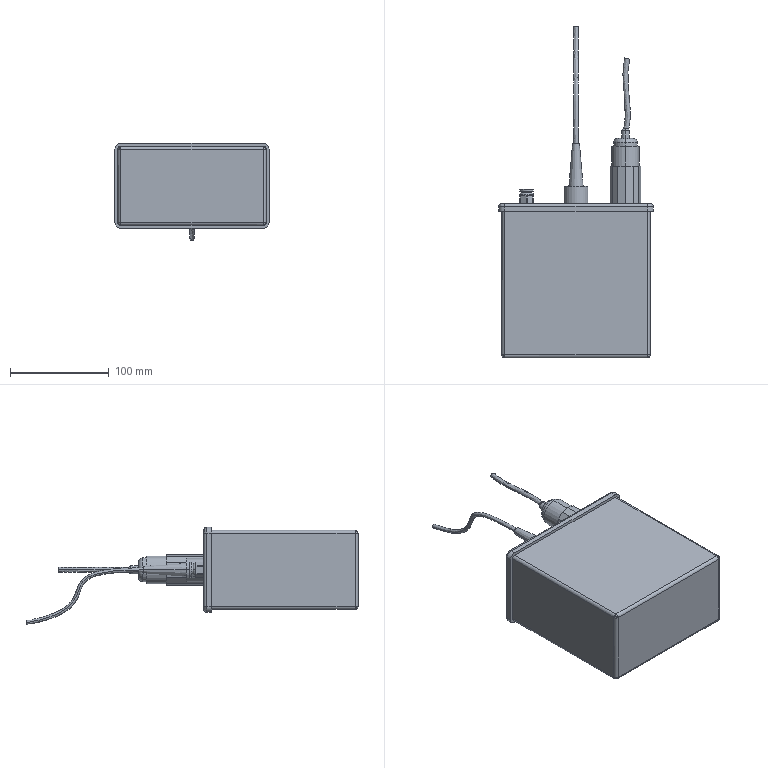Part | SolidWorks | 19 solids | 420 faces | box 156 x 335.859 x 98.479 mm | volume 1667612 mm3 | plane 189 | cylinder 163 | sphere 26 | spline 24 | torus 10 | cone 8 | commonest cylinder face diameters 6 x38 9.85 x14 8.141 x13 2 x12 7.779 x12 9.17 x12